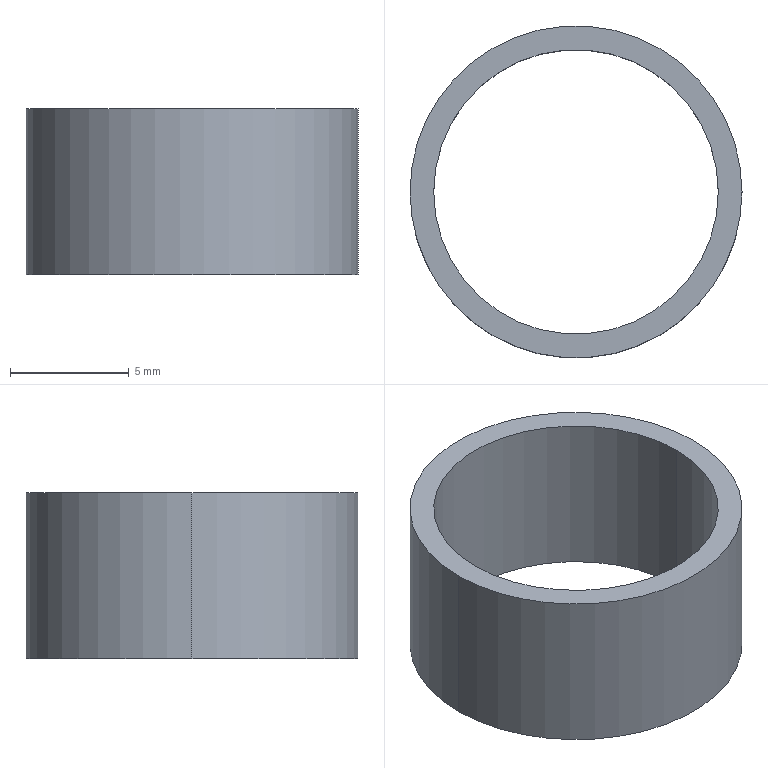Part | SolidWorks | features BaseBody 1 | 1 solid | 6 faces | box 14 x 14 x 7 mm | volume 285.885 mm3 | cylinder 4 | plane 2 | commonest cylinder face diameters 12 x2 14 x2
STEP:
#1=CARTESIAN_POINT('',(-6.,0.,3.5));
#2=VERTEX_POINT('',#1);
#3=CARTESIAN_POINT('',(6.,0.,3.5));
#4=VERTEX_POINT('',#3);
#5=CARTESIAN_POINT('',(0.,0.,3.5));
#6=DIRECTION('',(0.,0.,1.));
#7=DIRECTION('',(1.,0.,0.));
#8=AXIS2_PLACEMENT_3D('',#5,#6,#7);
#9=CIRCLE('',#8,6.);
#10=EDGE_CURVE('',#2,#4,#9,.T.);
#11=ORIENTED_EDGE('',*,*,#10,.T.);
#12=CARTESIAN_POINT('',(6.,0.,-3.5));
#13=VERTEX_POINT('',#12);
#14=CARTESIAN_POINT('',(6.,0.,3.5));
#15=DIRECTION('',(0.,0.,-1.));
#16=VECTOR('',#15,1000.);
#17=LINE('',#14,#16);
#18=EDGE_CURVE('',#4,#13,#17,.T.);
#19=ORIENTED_EDGE('',*,*,#18,.T.);
#20=CARTESIAN_POINT('',(-6.,0.,-3.5));
#21=VERTEX_POINT('',#20);
#22=CARTESIAN_POINT('',(0.,0.,-3.5));
#23=DIRECTION('',(0.,0.,1.));
#24=DIRECTION('',(1.,0.,0.));
#25=AXIS2_PLACEMENT_3D('',#22,#23,#24);
#26=CIRCLE('',#25,6.);
#27=EDGE_CURVE('',#21,#13,#26,.T.);
#28=ORIENTED_EDGE('',*,*,#27,.F.);
#29=CARTESIAN_POINT('',(-6.,0.,3.5));
#30=DIRECTION('',(0.,0.,-1.));
#31=VECTOR('',#30,1000.);
#32=LINE('',#29,#31);
#33=EDGE_CURVE('',#2,#21,#32,.T.);
#34=ORIENTED_EDGE('',*,*,#33,.F.);
#35=EDGE_LOOP('',(#11,#19,#28,#34));
#36=FACE_OUTER_BOUND('',#35,.T.);
#37=CARTESIAN_POINT('',(0.,0.,3.5));
#38=DIRECTION('',(0.,0.,-1.));
#39=DIRECTION('',(-1.,0.,0.));
#40=AXIS2_PLACEMENT_3D('',#37,#38,#39);
#41=CYLINDRICAL_SURFACE('',#40,6.);
#42=ADVANCED_FACE('',(#36),#41,.F.);
#43=CARTESIAN_POINT('',(7.,0.,3.5));
#44=VERTEX_POINT('',#43);
#45=CARTESIAN_POINT('',(-7.,0.,3.5));
#46=VERTEX_POINT('',#45);
#47=CARTESIAN_POINT('',(0.,0.,3.5));
#48=DIRECTION('',(0.,0.,1.));
#49=DIRECTION('',(1.,0.,0.));
#50=AXIS2_PLACEMENT_3D('',#47,#48,#49);
#51=CIRCLE('',#50,7.);
#52=EDGE_CURVE('',#44,#46,#51,.T.);
#53=ORIENTED_EDGE('',*,*,#52,.F.);
#54=CARTESIAN_POINT('',(7.,0.,-3.5));
#55=VERTEX_POINT('',#54);
#56=CARTESIAN_POINT('',(7.,0.,3.5));
#57=DIRECTION('',(0.,0.,-1.));
#58=VECTOR('',#57,1000.);
#59=LINE('',#56,#58);
#60=EDGE_CURVE('',#44,#55,#59,.T.);
#61=ORIENTED_EDGE('',*,*,#60,.T.);
#62=CARTESIAN_POINT('',(-7.,0.,-3.5));
#63=VERTEX_POINT('',#62);
#64=CARTESIAN_POINT('',(0.,0.,-3.5));
#65=DIRECTION('',(0.,0.,1.));
#66=DIRECTION('',(1.,0.,0.));
#67=AXIS2_PLACEMENT_3D('',#64,#65,#66);
#68=CIRCLE('',#67,7.);
#69=EDGE_CURVE('',#55,#63,#68,.T.);
#70=ORIENTED_EDGE('',*,*,#69,.T.);
#71=CARTESIAN_POINT('',(-7.,0.,3.5));
#72=DIRECTION('',(0.,0.,-1.));
#73=VECTOR('',#72,1000.);
#74=LINE('',#71,#73);
#75=EDGE_CURVE('',#46,#63,#74,.T.);
#76=ORIENTED_EDGE('',*,*,#75,.F.);
#77=EDGE_LOOP('',(#53,#61,#70,#76));
#78=FACE_OUTER_BOUND('',#77,.T.);
#79=CARTESIAN_POINT('',(0.,0.,3.5));
#80=DIRECTION('',(0.,0.,-1.));
#81=DIRECTION('',(-1.,0.,0.));
#82=AXIS2_PLACEMENT_3D('',#79,#80,#81);
#83=CYLINDRICAL_SURFACE('',#82,7.);
#84=ADVANCED_FACE('',(#78),#83,.T.);
#85=CARTESIAN_POINT('',(0.,0.,3.5));
#86=DIRECTION('',(0.,0.,1.));
#87=DIRECTION('',(1.,0.,0.));
#88=AXIS2_PLACEMENT_3D('',#85,#86,#87);
#89=CIRCLE('',#88,7.);
#90=EDGE_CURVE('',#46,#44,#89,.T.);
#91=ORIENTED_EDGE('',*,*,#90,.T.);
#92=ORIENTED_EDGE('',*,*,#52,.T.);
#93=EDGE_LOOP('',(#91,#92));
#94=FACE_OUTER_BOUND('',#93,.T.);
#95=ORIENTED_EDGE('',*,*,#10,.F.);
#96=CARTESIAN_POINT('',(0.,0.,3.5));
#97=DIRECTION('',(0.,0.,1.));
#98=DIRECTION('',(1.,0.,0.));
#99=AXIS2_PLACEMENT_3D('',#96,#97,#98);
#100=CIRCLE('',#99,6.);
#101=EDGE_CURVE('',#4,#2,#100,.T.);
#102=ORIENTED_EDGE('',*,*,#101,.F.);
#103=EDGE_LOOP('',(#95,#102));
#104=FACE_BOUND('',#103,.T.);
#105=CARTESIAN_POINT('',(0.,0.,3.5));
#106=DIRECTION('',(0.,0.,1.));
#107=DIRECTION('',(1.,0.,0.));
#108=AXIS2_PLACEMENT_3D('',#105,#106,#107);
#109=PLANE('',#108);
#110=ADVANCED_FACE('',(#94,#104),#109,.T.);
#111=CARTESIAN_POINT('',(0.,0.,-3.5));
#112=DIRECTION('',(0.,0.,1.));
#113=DIRECTION('',(1.,0.,0.));
#114=AXIS2_PLACEMENT_3D('',#111,#112,#113);
#115=CIRCLE('',#114,7.);
#116=EDGE_CURVE('',#63,#55,#115,.T.);
#117=ORIENTED_EDGE('',*,*,#116,.F.);
#118=ORIENTED_EDGE('',*,*,#69,.F.);
#119=EDGE_LOOP('',(#117,#118));
#120=FACE_OUTER_BOUND('',#119,.T.);
#121=ORIENTED_EDGE('',*,*,#27,.T.);
#122=CARTESIAN_POINT('',(0.,0.,-3.5));
#123=DIRECTION('',(0.,0.,1.));
#124=DIRECTION('',(1.,0.,0.));
#125=AXIS2_PLACEMENT_3D('',#122,#123,#124);
#126=CIRCLE('',#125,6.);
#127=EDGE_CURVE('',#13,#21,#126,.T.);
#128=ORIENTED_EDGE('',*,*,#127,.T.);
#129=EDGE_LOOP('',(#121,#128));
#130=FACE_BOUND('',#129,.T.);
#131=CARTESIAN_POINT('',(0.,0.,-3.5));
#132=DIRECTION('',(0.,0.,1.));
#133=DIRECTION('',(1.,0.,0.));
#134=AXIS2_PLACEMENT_3D('',#131,#132,#133);
#135=PLANE('',#134);
#136=ADVANCED_FACE('',(#120,#130),#135,.F.);
#137=ORIENTED_EDGE('',*,*,#60,.F.);
#138=ORIENTED_EDGE('',*,*,#90,.F.);
#139=ORIENTED_EDGE('',*,*,#75,.T.);
#140=ORIENTED_EDGE('',*,*,#116,.T.);
#141=EDGE_LOOP('',(#137,#138,#139,#140));
#142=FACE_OUTER_BOUND('',#141,.T.);
#143=CARTESIAN_POINT('',(0.,0.,3.5));
#144=DIRECTION('',(0.,0.,-1.));
#145=DIRECTION('',(-1.,0.,0.));
#146=AXIS2_PLACEMENT_3D('',#143,#144,#145);
#147=CYLINDRICAL_SURFACE('',#146,7.);
#148=ADVANCED_FACE('',(#142),#147,.T.);
#149=ORIENTED_EDGE('',*,*,#18,.F.);
#150=ORIENTED_EDGE('',*,*,#101,.T.);
#151=ORIENTED_EDGE('',*,*,#33,.T.);
#152=ORIENTED_EDGE('',*,*,#127,.F.);
#153=EDGE_LOOP('',(#149,#150,#151,#152));
#154=FACE_OUTER_BOUND('',#153,.T.);
#155=CARTESIAN_POINT('',(0.,0.,3.5));
#156=DIRECTION('',(0.,0.,-1.));
#157=DIRECTION('',(-1.,0.,0.));
#158=AXIS2_PLACEMENT_3D('',#155,#156,#157);
#159=CYLINDRICAL_SURFACE('',#158,6.);
#160=ADVANCED_FACE('',(#154),#159,.F.);
#161=CLOSED_SHELL('',(#42,#84,#110,#136,#148,#160));
#162=MANIFOLD_SOLID_BREP('',#161);
#163=CARTESIAN_POINT('',(0.,0.,0.));
#164=DIRECTION('',(0.,0.,1.));
#165=DIRECTION('',(1.,0.,0.));
#166=AXIS2_PLACEMENT_3D('',#163,#164,#165);
#167=(LENGTH_UNIT()NAMED_UNIT(*)SI_UNIT(.MILLI.,.METRE.));
#168=UNCERTAINTY_MEASURE_WITH_UNIT(LENGTH_MEASURE(0.00001),#167,'','');
#169=(NAMED_UNIT(*)PLANE_ANGLE_UNIT()SI_UNIT($,.RADIAN.));
#170=(NAMED_UNIT(*)SI_UNIT($,.STERADIAN.)SOLID_ANGLE_UNIT());
#171=(GEOMETRIC_REPRESENTATION_CONTEXT(3)GLOBAL_UNCERTAINTY_ASSIGNED_CONTEXT((#168))GLOBAL_UNIT_ASSIGNED_CONTEXT((#167,#169,#170))REPRESENTATION_CONTEXT('',''));
#172=ADVANCED_BREP_SHAPE_REPRESENTATION('',(#162,#166),#171);